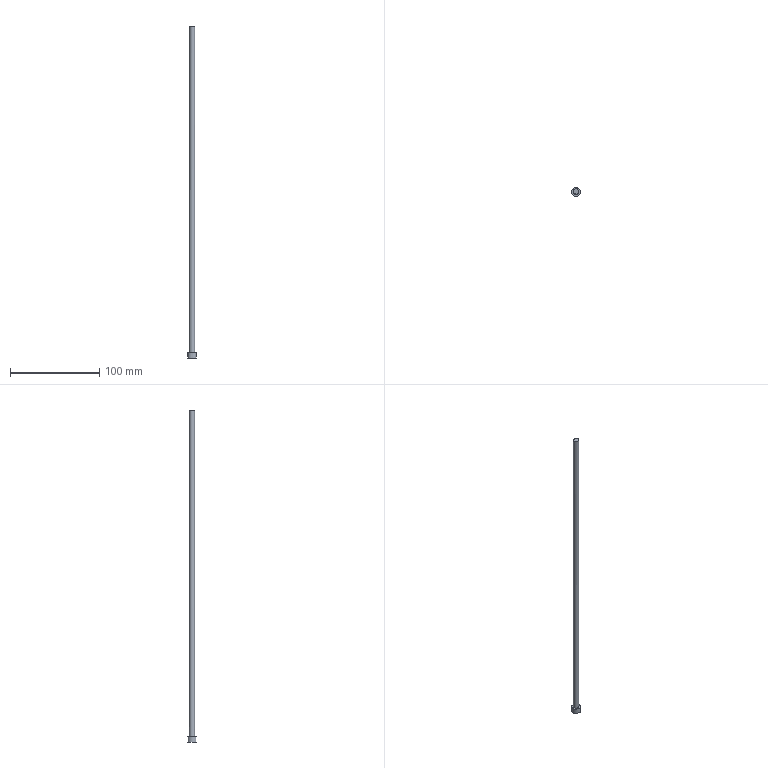Part | NX | features solid 2 | 1 solid | 5 faces | box 10 x 10 x 372.984 mm | volume 10833 mm3 | cylinder 2 | plane 2 | spline 1 | commonest cylinder face diameters 6 x1 10 x1
STEP:
#1=CARTESIAN_POINT('',(56.,69.,-339.5));
#2=VERTEX_POINT('',#1);
#3=CARTESIAN_POINT('',(59.,69.,-339.5));
#4=DIRECTION('',(0.,0.,-1.));
#5=DIRECTION('',(-1.,0.,0.));
#6=AXIS2_PLACEMENT_3D('',#3,#4,#5);
#7=CIRCLE('',#6,3.);
#8=EDGE_CURVE('',#2,#2,#7,.T.);
#9=ORIENTED_EDGE('',*,*,#8,.F.);
#10=EDGE_LOOP('',(#9));
#11=FACE_BOUND('',#10,.T.);
#12=CARTESIAN_POINT('',(56.017,68.677,26.641));
#13=VERTEX_POINT('',#12);
#14=CARTESIAN_POINT('',(56.926,66.404,26.799));
#15=CARTESIAN_POINT('',(55.69,68.641,26.595));
#16=CARTESIAN_POINT('',(56.419,71.098,26.669));
#17=CARTESIAN_POINT('',(58.649,72.301,26.971));
#18=CARTESIAN_POINT('',(61.076,71.595,27.322));
#19=CARTESIAN_POINT('',(62.309,69.36,27.522));
#20=CARTESIAN_POINT('',(61.584,66.906,27.45));
#21=CARTESIAN_POINT('',(59.351,65.698,27.151));
#22=CARTESIAN_POINT('',(56.926,66.404,26.799));
#23=CARTESIAN_POINT('',(55.69,68.641,26.595));
#24=CARTESIAN_POINT('',(56.419,71.098,26.669));
#25=B_SPLINE_CURVE_WITH_KNOTS('',3,(#14,#15,#16,#17,#18,#19,#20,#21,#22,#23,#24),.UNSPECIFIED.,.T.,.F.,(1,1,1,1,1,1,1,1,1,1,1,1,1,1,1),(-0.00707,-0.004713,-0.002357,0.,0.002357,0.004713,0.00707,0.009426,0.01178,0.01414,0.0165,0.01885,0.02121,0.02357,0.02592),.UNSPECIFIED.);
#26=EDGE_CURVE('',#13,#13,#25,.T.);
#27=ORIENTED_EDGE('',*,*,#26,.T.);
#28=EDGE_LOOP('',(#27));
#29=FACE_BOUND('',#28,.T.);
#30=CARTESIAN_POINT('',(59.,69.,-345.5));
#31=DIRECTION('',(0.,0.,1.));
#32=DIRECTION('',(-1.,0.,0.));
#33=AXIS2_PLACEMENT_3D('',#30,#31,#32);
#34=CYLINDRICAL_SURFACE('',#33,3.);
#35=ADVANCED_FACE('',(#11,#29),#34,.T.);
#36=ORIENTED_EDGE('',*,*,#8,.T.);
#37=EDGE_LOOP('',(#36));
#38=FACE_BOUND('',#37,.T.);
#39=CARTESIAN_POINT('',(54.,69.,-339.5));
#40=VERTEX_POINT('',#39);
#41=CARTESIAN_POINT('',(59.,69.,-339.5));
#42=DIRECTION('',(0.,0.,1.));
#43=DIRECTION('',(-1.,0.,0.));
#44=AXIS2_PLACEMENT_3D('',#41,#42,#43);
#45=CIRCLE('',#44,5.);
#46=EDGE_CURVE('',#40,#40,#45,.T.);
#47=ORIENTED_EDGE('',*,*,#46,.T.);
#48=EDGE_LOOP('',(#47));
#49=FACE_BOUND('',#48,.T.);
#50=CARTESIAN_POINT('',(59.,69.,-339.5));
#51=DIRECTION('',(0.,0.,1.));
#52=DIRECTION('',(-1.,0.,0.));
#53=AXIS2_PLACEMENT_3D('',#50,#51,#52);
#54=PLANE('',#53);
#55=ADVANCED_FACE('',(#38,#49),#54,.T.);
#56=CARTESIAN_POINT('',(54.,69.,-345.5));
#57=VERTEX_POINT('',#56);
#58=CARTESIAN_POINT('',(59.,69.,-345.5));
#59=DIRECTION('',(0.,0.,-1.));
#60=DIRECTION('',(-1.,0.,0.));
#61=AXIS2_PLACEMENT_3D('',#58,#59,#60);
#62=CIRCLE('',#61,5.);
#63=EDGE_CURVE('',#57,#57,#62,.T.);
#64=ORIENTED_EDGE('',*,*,#63,.T.);
#65=EDGE_LOOP('',(#64));
#66=FACE_BOUND('',#65,.T.);
#67=CARTESIAN_POINT('',(59.,69.,-345.5));
#68=DIRECTION('',(0.,0.,-1.));
#69=DIRECTION('',(1.,0.,0.));
#70=AXIS2_PLACEMENT_3D('',#67,#68,#69);
#71=PLANE('',#70);
#72=ADVANCED_FACE('',(#66),#71,.T.);
#73=ORIENTED_EDGE('',*,*,#46,.F.);
#74=EDGE_LOOP('',(#73));
#75=FACE_BOUND('',#74,.T.);
#76=ORIENTED_EDGE('',*,*,#63,.F.);
#77=EDGE_LOOP('',(#76));
#78=FACE_BOUND('',#77,.T.);
#79=CARTESIAN_POINT('',(59.,69.,-345.5));
#80=DIRECTION('',(0.,0.,1.));
#81=DIRECTION('',(-1.,0.,0.));
#82=AXIS2_PLACEMENT_3D('',#79,#80,#81);
#83=CYLINDRICAL_SURFACE('',#82,5.);
#84=ADVANCED_FACE('',(#75,#78),#83,.T.);
#85=ORIENTED_EDGE('',*,*,#26,.F.);
#86=EDGE_LOOP('',(#85));
#87=FACE_BOUND('',#86,.T.);
#88=CARTESIAN_POINT('',(55.942,65.944,26.666));
#89=CARTESIAN_POINT('',(55.944,67.975,26.639));
#90=CARTESIAN_POINT('',(55.947,70.006,26.614));
#91=CARTESIAN_POINT('',(55.949,72.036,26.592));
#92=CARTESIAN_POINT('',(57.978,65.945,26.954));
#93=CARTESIAN_POINT('',(57.98,67.975,26.927));
#94=CARTESIAN_POINT('',(57.983,70.006,26.902));
#95=CARTESIAN_POINT('',(57.985,72.037,26.88));
#96=CARTESIAN_POINT('',(60.015,65.945,27.241));
#97=CARTESIAN_POINT('',(60.017,67.976,27.215));
#98=CARTESIAN_POINT('',(60.019,70.007,27.19));
#99=CARTESIAN_POINT('',(60.021,72.038,27.168));
#100=CARTESIAN_POINT('',(62.052,65.946,27.529));
#101=CARTESIAN_POINT('',(62.054,67.977,27.502));
#102=CARTESIAN_POINT('',(62.055,70.007,27.478));
#103=CARTESIAN_POINT('',(62.057,72.038,27.456));
#104=B_SPLINE_SURFACE_WITH_KNOTS('',3,3,((#88,#89,#90,#91),(#92,#93,#94,#95),(#96,#97,#98,#99),(#100,#101,#102,#103)),.UNSPECIFIED.,.F.,.F.,.F.,(4,4),(4,4),(0.9321,0.963),(0.8036,0.9192),.PIECEWISE_BEZIER_KNOTS.);
#105=ADVANCED_FACE('',(#87),#104,.T.);
#106=CLOSED_SHELL('',(#35,#55,#72,#84,#105));
#107=MANIFOLD_SOLID_BREP('',#106);
#108=(LENGTH_UNIT()NAMED_UNIT(*)SI_UNIT(.MILLI.,.METRE.));
#109=UNCERTAINTY_MEASURE_WITH_UNIT(LENGTH_MEASURE(0.0508),#108,'','');
#110=(NAMED_UNIT(*)PLANE_ANGLE_UNIT()SI_UNIT($,.RADIAN.));
#111=(NAMED_UNIT(*)SI_UNIT($,.STERADIAN.)SOLID_ANGLE_UNIT());
#112=(GEOMETRIC_REPRESENTATION_CONTEXT(3)GLOBAL_UNCERTAINTY_ASSIGNED_CONTEXT((#109))GLOBAL_UNIT_ASSIGNED_CONTEXT((#108,#110,#111))REPRESENTATION_CONTEXT('',''));
#113=ADVANCED_BREP_SHAPE_REPRESENTATION('',(#107),#112);